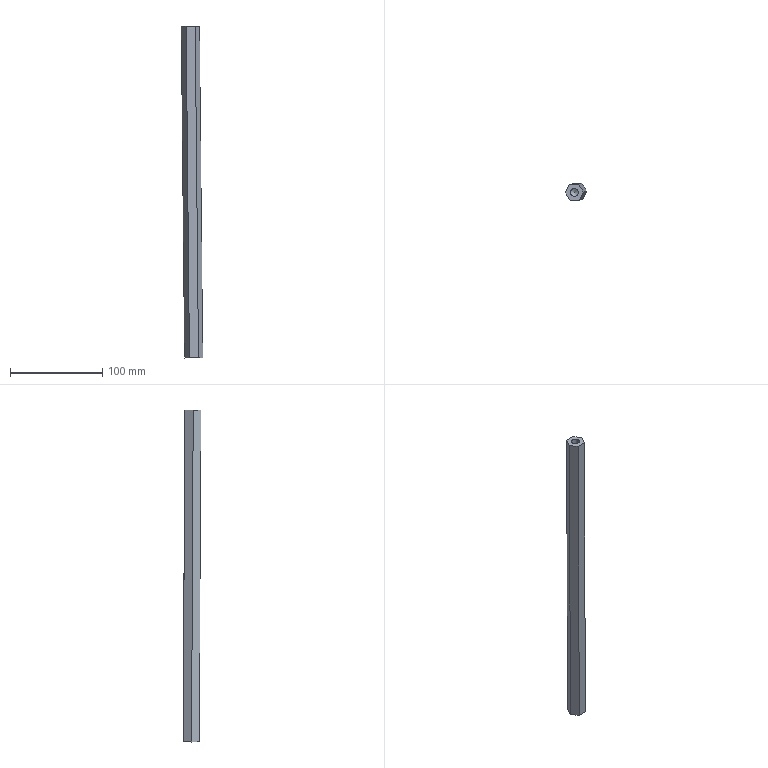Part | NX | features A0 2 | 1 solid | 12 faces | box 23.181 x 19.188 x 360.176 mm | volume 87224 mm3 | plane 8 | cone 2 | cylinder 2 | commonest cylinder face diameters 8.5 x2
STEP:
#1=CARTESIAN_POINT('',(-114.316,94.668,-584.763));
#2=VERTEX_POINT('',#1);
#3=CARTESIAN_POINT('',(-110.07,94.842,-584.72));
#4=DIRECTION('',(0.009912,0.004999,-0.9999));
#5=DIRECTION('',(-0.9991,-0.04102,-0.01011));
#6=AXIS2_PLACEMENT_3D('',#3,#4,#5);
#7=CIRCLE('',#6,4.25);
#8=EDGE_CURVE('',#2,#2,#7,.T.);
#9=ORIENTED_EDGE('',*,*,#8,.T.);
#10=EDGE_LOOP('',(#9));
#11=FACE_BOUND('',#10,.T.);
#12=CARTESIAN_POINT('',(-110.095,94.829,-582.166));
#13=VERTEX_POINT('',#12);
#14=VERTEX_LOOP('',#13);
#15=FACE_BOUND('',#14,.T.);
#16=CARTESIAN_POINT('',(-110.095,94.829,-582.166));
#17=DIRECTION('',(0.009912,0.004999,-0.9999));
#18=DIRECTION('',(-0.9991,-0.04102,-0.01011));
#19=AXIS2_PLACEMENT_3D('',#16,#17,#18);
#20=CONICAL_SURFACE('',#19,0.,1.03);
#21=ADVANCED_FACE('',(#11,#15),#20,.F.);
#22=CARTESIAN_POINT('',(-105.581,95.139,-609.175));
#23=VERTEX_POINT('',#22);
#24=CARTESIAN_POINT('',(-109.827,94.964,-609.218));
#25=DIRECTION('',(-0.009912,-0.004999,0.9999));
#26=DIRECTION('',(0.9991,0.04102,0.01011));
#27=AXIS2_PLACEMENT_3D('',#24,#25,#26);
#28=CIRCLE('',#27,4.25);
#29=EDGE_CURVE('',#23,#23,#28,.T.);
#30=ORIENTED_EDGE('',*,*,#29,.F.);
#31=EDGE_LOOP('',(#30));
#32=FACE_BOUND('',#31,.T.);
#33=ORIENTED_EDGE('',*,*,#8,.F.);
#34=EDGE_LOOP('',(#33));
#35=FACE_BOUND('',#34,.T.);
#36=CARTESIAN_POINT('',(-109.827,94.964,-609.218));
#37=DIRECTION('',(0.009912,0.004999,-0.9999));
#38=DIRECTION('',(-0.9991,-0.04102,-0.01011));
#39=AXIS2_PLACEMENT_3D('',#36,#37,#38);
#40=CYLINDRICAL_SURFACE('',#39,4.25);
#41=ADVANCED_FACE('',(#32,#35),#40,.F.);
#42=ORIENTED_EDGE('',*,*,#29,.T.);
#43=EDGE_LOOP('',(#42));
#44=FACE_BOUND('',#43,.T.);
#45=CARTESIAN_POINT('',(-119.633,94.562,-609.318));
#46=VERTEX_POINT('',#45);
#47=CARTESIAN_POINT('',(-115.079,103.256,-609.229));
#48=VERTEX_POINT('',#47);
#49=CARTESIAN_POINT('',(-119.633,94.562,-609.318));
#50=DIRECTION('',(0.464,0.8858,0.009027));
#51=VECTOR('',#50,1000.);
#52=LINE('',#49,#51);
#53=EDGE_CURVE('',#46,#48,#52,.T.);
#54=ORIENTED_EDGE('',*,*,#53,.T.);
#55=CARTESIAN_POINT('',(-105.273,103.659,-609.13));
#56=VERTEX_POINT('',#55);
#57=CARTESIAN_POINT('',(-105.273,103.659,-609.13));
#58=DIRECTION('',(-0.9991,-0.04102,-0.01011));
#59=VECTOR('',#58,1000.);
#60=LINE('',#57,#59);
#61=EDGE_CURVE('',#56,#48,#60,.T.);
#62=ORIENTED_EDGE('',*,*,#61,.F.);
#63=CARTESIAN_POINT('',(-100.021,95.367,-609.119));
#64=VERTEX_POINT('',#63);
#65=CARTESIAN_POINT('',(-105.273,103.659,-609.13));
#66=DIRECTION('',(0.5351,-0.8448,0.001081));
#67=VECTOR('',#66,1000.);
#68=LINE('',#65,#67);
#69=EDGE_CURVE('',#56,#64,#68,.T.);
#70=ORIENTED_EDGE('',*,*,#69,.T.);
#71=CARTESIAN_POINT('',(-104.575,86.673,-609.208));
#72=VERTEX_POINT('',#71);
#73=CARTESIAN_POINT('',(-100.021,95.367,-609.119));
#74=DIRECTION('',(-0.464,-0.8858,-0.009027));
#75=VECTOR('',#74,1000.);
#76=LINE('',#73,#75);
#77=EDGE_CURVE('',#64,#72,#76,.T.);
#78=ORIENTED_EDGE('',*,*,#77,.T.);
#79=CARTESIAN_POINT('',(-114.381,86.27,-609.307));
#80=VERTEX_POINT('',#79);
#81=CARTESIAN_POINT('',(-114.381,86.27,-609.307));
#82=DIRECTION('',(0.9991,0.04102,0.01011));
#83=VECTOR('',#82,1000.);
#84=LINE('',#81,#83);
#85=EDGE_CURVE('',#80,#72,#84,.T.);
#86=ORIENTED_EDGE('',*,*,#85,.F.);
#87=CARTESIAN_POINT('',(-114.381,86.27,-609.307));
#88=DIRECTION('',(-0.5351,0.8448,-0.001081));
#89=VECTOR('',#88,1000.);
#90=LINE('',#87,#89);
#91=EDGE_CURVE('',#80,#46,#90,.T.);
#92=ORIENTED_EDGE('',*,*,#91,.T.);
#93=EDGE_LOOP('',(#54,#62,#70,#78,#86,#92));
#94=FACE_BOUND('',#93,.T.);
#95=CARTESIAN_POINT('',(-109.827,94.964,-609.218));
#96=DIRECTION('',(0.009912,0.004999,-0.9999));
#97=DIRECTION('',(-0.9991,-0.04102,-0.01011));
#98=AXIS2_PLACEMENT_3D('',#95,#96,#97);
#99=PLANE('',#98);
#100=ADVANCED_FACE('',(#44,#94),#99,.T.);
#101=CARTESIAN_POINT('',(-118.647,101.456,-249.251));
#102=VERTEX_POINT('',#101);
#103=CARTESIAN_POINT('',(-118.647,101.456,-249.251));
#104=DIRECTION('',(0.009912,0.004999,-0.9999));
#105=VECTOR('',#104,1000.);
#106=LINE('',#103,#105);
#107=EDGE_CURVE('',#102,#48,#106,.T.);
#108=ORIENTED_EDGE('',*,*,#107,.T.);
#109=ORIENTED_EDGE('',*,*,#53,.F.);
#110=CARTESIAN_POINT('',(-123.201,92.762,-249.34));
#111=VERTEX_POINT('',#110);
#112=CARTESIAN_POINT('',(-123.201,92.762,-249.34));
#113=DIRECTION('',(0.009912,0.004999,-0.9999));
#114=VECTOR('',#113,1000.);
#115=LINE('',#112,#114);
#116=EDGE_CURVE('',#111,#46,#115,.T.);
#117=ORIENTED_EDGE('',*,*,#116,.F.);
#118=CARTESIAN_POINT('',(-118.647,101.456,-249.251));
#119=DIRECTION('',(-0.464,-0.8858,-0.009027));
#120=VECTOR('',#119,1000.);
#121=LINE('',#118,#120);
#122=EDGE_CURVE('',#102,#111,#121,.T.);
#123=ORIENTED_EDGE('',*,*,#122,.F.);
#124=EDGE_LOOP('',(#108,#109,#117,#123));
#125=FACE_BOUND('',#124,.T.);
#126=CARTESIAN_POINT('',(-119.633,94.562,-609.318));
#127=DIRECTION('',(0.8858,-0.464,0.00646));
#128=DIRECTION('',(-0.464,-0.8858,-0.009027));
#129=AXIS2_PLACEMENT_3D('',#126,#127,#128);
#130=PLANE('',#129);
#131=ADVANCED_FACE('',(#125),#130,.F.);
#132=CARTESIAN_POINT('',(-108.841,101.859,-249.152));
#133=VERTEX_POINT('',#132);
#134=CARTESIAN_POINT('',(-108.841,101.859,-249.152));
#135=DIRECTION('',(0.009912,0.004999,-0.9999));
#136=VECTOR('',#135,1000.);
#137=LINE('',#134,#136);
#138=EDGE_CURVE('',#133,#56,#137,.T.);
#139=ORIENTED_EDGE('',*,*,#138,.T.);
#140=ORIENTED_EDGE('',*,*,#61,.T.);
#141=ORIENTED_EDGE('',*,*,#107,.F.);
#142=CARTESIAN_POINT('',(-108.841,101.859,-249.152));
#143=DIRECTION('',(-0.9991,-0.04102,-0.01011));
#144=VECTOR('',#143,1000.);
#145=LINE('',#142,#144);
#146=EDGE_CURVE('',#133,#102,#145,.T.);
#147=ORIENTED_EDGE('',*,*,#146,.F.);
#148=EDGE_LOOP('',(#139,#140,#141,#147));
#149=FACE_BOUND('',#148,.T.);
#150=CARTESIAN_POINT('',(-115.079,103.256,-609.229));
#151=DIRECTION('',(0.04107,-0.9991,-0.004588));
#152=DIRECTION('',(-0.9991,-0.04102,-0.01011));
#153=AXIS2_PLACEMENT_3D('',#150,#151,#152);
#154=PLANE('',#153);
#155=ADVANCED_FACE('',(#149),#154,.F.);
#156=CARTESIAN_POINT('',(-103.589,93.568,-249.141));
#157=VERTEX_POINT('',#156);
#158=CARTESIAN_POINT('',(-103.589,93.568,-249.141));
#159=DIRECTION('',(0.009912,0.004999,-0.9999));
#160=VECTOR('',#159,1000.);
#161=LINE('',#158,#160);
#162=EDGE_CURVE('',#157,#64,#161,.T.);
#163=ORIENTED_EDGE('',*,*,#162,.T.);
#164=ORIENTED_EDGE('',*,*,#69,.F.);
#165=ORIENTED_EDGE('',*,*,#138,.F.);
#166=CARTESIAN_POINT('',(-103.589,93.568,-249.141));
#167=DIRECTION('',(-0.5351,0.8448,-0.001081));
#168=VECTOR('',#167,1000.);
#169=LINE('',#166,#168);
#170=EDGE_CURVE('',#157,#133,#169,.T.);
#171=ORIENTED_EDGE('',*,*,#170,.F.);
#172=EDGE_LOOP('',(#163,#164,#165,#171));
#173=FACE_BOUND('',#172,.T.);
#174=CARTESIAN_POINT('',(-105.273,103.659,-609.13));
#175=DIRECTION('',(-0.8447,-0.5351,-0.01105));
#176=DIRECTION('',(-0.5351,0.8448,-0.001081));
#177=AXIS2_PLACEMENT_3D('',#174,#175,#176);
#178=PLANE('',#177);
#179=ADVANCED_FACE('',(#173),#178,.F.);
#180=CARTESIAN_POINT('',(-108.143,84.874,-249.23));
#181=VERTEX_POINT('',#180);
#182=CARTESIAN_POINT('',(-108.143,84.874,-249.23));
#183=DIRECTION('',(0.009912,0.004999,-0.9999));
#184=VECTOR('',#183,1000.);
#185=LINE('',#182,#184);
#186=EDGE_CURVE('',#181,#72,#185,.T.);
#187=ORIENTED_EDGE('',*,*,#186,.T.);
#188=ORIENTED_EDGE('',*,*,#77,.F.);
#189=ORIENTED_EDGE('',*,*,#162,.F.);
#190=CARTESIAN_POINT('',(-108.143,84.874,-249.23));
#191=DIRECTION('',(0.464,0.8858,0.009027));
#192=VECTOR('',#191,1000.);
#193=LINE('',#190,#192);
#194=EDGE_CURVE('',#181,#157,#193,.T.);
#195=ORIENTED_EDGE('',*,*,#194,.F.);
#196=EDGE_LOOP('',(#187,#188,#189,#195));
#197=FACE_BOUND('',#196,.T.);
#198=CARTESIAN_POINT('',(-100.021,95.367,-609.119));
#199=DIRECTION('',(-0.8858,0.464,-0.00646));
#200=DIRECTION('',(0.464,0.8858,0.009027));
#201=AXIS2_PLACEMENT_3D('',#198,#199,#200);
#202=PLANE('',#201);
#203=ADVANCED_FACE('',(#197),#202,.F.);
#204=CARTESIAN_POINT('',(-117.949,84.471,-249.329));
#205=VERTEX_POINT('',#204);
#206=CARTESIAN_POINT('',(-117.949,84.471,-249.329));
#207=DIRECTION('',(0.009912,0.004999,-0.9999));
#208=VECTOR('',#207,1000.);
#209=LINE('',#206,#208);
#210=EDGE_CURVE('',#205,#80,#209,.T.);
#211=ORIENTED_EDGE('',*,*,#210,.T.);
#212=ORIENTED_EDGE('',*,*,#85,.T.);
#213=ORIENTED_EDGE('',*,*,#186,.F.);
#214=CARTESIAN_POINT('',(-117.949,84.471,-249.329));
#215=DIRECTION('',(0.9991,0.04102,0.01011));
#216=VECTOR('',#215,1000.);
#217=LINE('',#214,#216);
#218=EDGE_CURVE('',#205,#181,#217,.T.);
#219=ORIENTED_EDGE('',*,*,#218,.F.);
#220=EDGE_LOOP('',(#211,#212,#213,#219));
#221=FACE_BOUND('',#220,.T.);
#222=CARTESIAN_POINT('',(-104.575,86.673,-609.208));
#223=DIRECTION('',(-0.04107,0.9991,0.004588));
#224=DIRECTION('',(0.009912,0.004999,-0.9999));
#225=AXIS2_PLACEMENT_3D('',#222,#223,#224);
#226=PLANE('',#225);
#227=ADVANCED_FACE('',(#221),#226,.F.);
#228=ORIENTED_EDGE('',*,*,#116,.T.);
#229=ORIENTED_EDGE('',*,*,#91,.F.);
#230=ORIENTED_EDGE('',*,*,#210,.F.);
#231=CARTESIAN_POINT('',(-123.201,92.762,-249.34));
#232=DIRECTION('',(0.5351,-0.8448,0.001081));
#233=VECTOR('',#232,1000.);
#234=LINE('',#231,#233);
#235=EDGE_CURVE('',#111,#205,#234,.T.);
#236=ORIENTED_EDGE('',*,*,#235,.F.);
#237=EDGE_LOOP('',(#228,#229,#230,#236));
#238=FACE_BOUND('',#237,.T.);
#239=CARTESIAN_POINT('',(-114.381,86.27,-609.307));
#240=DIRECTION('',(0.8447,0.5351,0.01105));
#241=DIRECTION('',(0.5351,-0.8448,0.001081));
#242=AXIS2_PLACEMENT_3D('',#239,#240,#241);
#243=PLANE('',#242);
#244=ADVANCED_FACE('',(#238),#243,.F.);
#245=CARTESIAN_POINT('',(-109.149,93.339,-249.198));
#246=VERTEX_POINT('',#245);
#247=CARTESIAN_POINT('',(-113.395,93.165,-249.241));
#248=DIRECTION('',(0.009912,0.004999,-0.9999));
#249=DIRECTION('',(0.9991,0.04102,0.01011));
#250=AXIS2_PLACEMENT_3D('',#247,#248,#249);
#251=CIRCLE('',#250,4.25);
#252=EDGE_CURVE('',#246,#246,#251,.T.);
#253=ORIENTED_EDGE('',*,*,#252,.T.);
#254=EDGE_LOOP('',(#253));
#255=FACE_BOUND('',#254,.T.);
#256=ORIENTED_EDGE('',*,*,#218,.T.);
#257=ORIENTED_EDGE('',*,*,#194,.T.);
#258=ORIENTED_EDGE('',*,*,#170,.T.);
#259=ORIENTED_EDGE('',*,*,#146,.T.);
#260=ORIENTED_EDGE('',*,*,#122,.T.);
#261=ORIENTED_EDGE('',*,*,#235,.T.);
#262=EDGE_LOOP('',(#256,#257,#258,#259,#260,#261));
#263=FACE_BOUND('',#262,.T.);
#264=CARTESIAN_POINT('',(-113.395,93.165,-249.241));
#265=DIRECTION('',(0.009912,0.004999,-0.9999));
#266=DIRECTION('',(-0.9991,-0.04102,-0.01011));
#267=AXIS2_PLACEMENT_3D('',#264,#265,#266);
#268=PLANE('',#267);
#269=ADVANCED_FACE('',(#255,#263),#268,.F.);
#270=CARTESIAN_POINT('',(-113.127,93.3,-276.293));
#271=VERTEX_POINT('',#270);
#272=VERTEX_LOOP('',#271);
#273=FACE_BOUND('',#272,.T.);
#274=CARTESIAN_POINT('',(-117.399,93.113,-273.782));
#275=VERTEX_POINT('',#274);
#276=CARTESIAN_POINT('',(-113.152,93.287,-273.739));
#277=DIRECTION('',(-0.009912,-0.004999,0.9999));
#278=DIRECTION('',(-0.9991,-0.04102,-0.01011));
#279=AXIS2_PLACEMENT_3D('',#276,#277,#278);
#280=CIRCLE('',#279,4.25);
#281=EDGE_CURVE('',#275,#275,#280,.T.);
#282=ORIENTED_EDGE('',*,*,#281,.T.);
#283=EDGE_LOOP('',(#282));
#284=FACE_BOUND('',#283,.T.);
#285=CARTESIAN_POINT('',(-113.127,93.3,-276.293));
#286=DIRECTION('',(-0.009912,-0.004999,0.9999));
#287=DIRECTION('',(0.9991,0.04102,0.01011));
#288=AXIS2_PLACEMENT_3D('',#285,#286,#287);
#289=CONICAL_SURFACE('',#288,0.,1.03);
#290=ADVANCED_FACE('',(#273,#284),#289,.F.);
#291=ORIENTED_EDGE('',*,*,#281,.F.);
#292=EDGE_LOOP('',(#291));
#293=FACE_BOUND('',#292,.T.);
#294=ORIENTED_EDGE('',*,*,#252,.F.);
#295=EDGE_LOOP('',(#294));
#296=FACE_BOUND('',#295,.T.);
#297=CARTESIAN_POINT('',(-113.395,93.165,-249.241));
#298=DIRECTION('',(-0.009912,-0.004999,0.9999));
#299=DIRECTION('',(0.9991,0.04102,0.01011));
#300=AXIS2_PLACEMENT_3D('',#297,#298,#299);
#301=CYLINDRICAL_SURFACE('',#300,4.25);
#302=ADVANCED_FACE('',(#293,#296),#301,.F.);
#303=CLOSED_SHELL('',(#21,#41,#100,#131,#155,#179,#203,#227,#244,#269,#290,#302));
#304=MANIFOLD_SOLID_BREP('',#303);
#305=(LENGTH_UNIT()NAMED_UNIT(*)SI_UNIT(.MILLI.,.METRE.));
#306=UNCERTAINTY_MEASURE_WITH_UNIT(LENGTH_MEASURE(0.00001),#305,'','');
#307=(NAMED_UNIT(*)PLANE_ANGLE_UNIT()SI_UNIT($,.RADIAN.));
#308=(NAMED_UNIT(*)SI_UNIT($,.STERADIAN.)SOLID_ANGLE_UNIT());
#309=(GEOMETRIC_REPRESENTATION_CONTEXT(3)GLOBAL_UNCERTAINTY_ASSIGNED_CONTEXT((#306))GLOBAL_UNIT_ASSIGNED_CONTEXT((#305,#307,#308))REPRESENTATION_CONTEXT('',''));
#310=ADVANCED_BREP_SHAPE_REPRESENTATION('',(#304),#309);